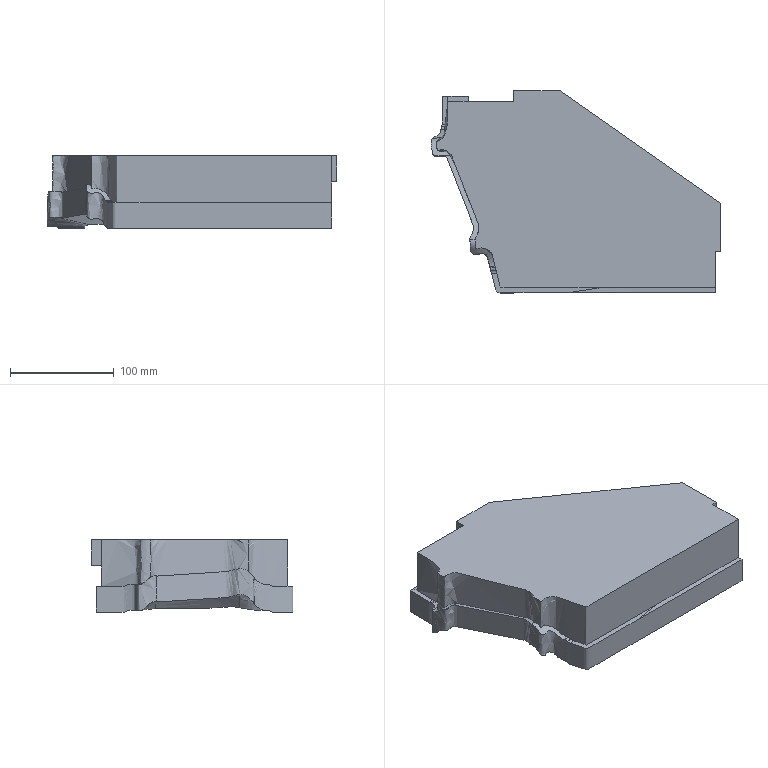Part | NX | features solid 2 | 1 solid | 56 faces | box 279.555 x 195.049 x 70.236 mm | volume 1418227 mm3 | spline 33 | plane 17 | cylinder 6 | commonest cylinder face diameters 30 x4 20 x1 25 x1